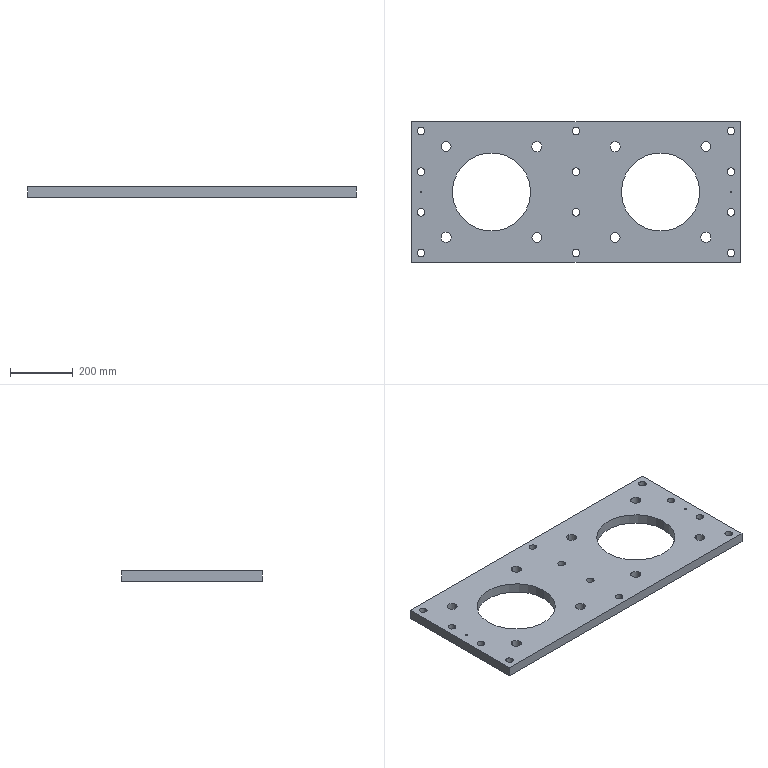Part | SolidWorks | features ICE 3, MirrorPattern 3, CirPattern 1, Extrusion 1, HoleWzd 1 | 1 solid | 54 faces | box 1050 x 450 x 32 mm | volume 11596993 mm3 | cylinder 48 | plane 6 | commonest cylinder face diameters 24 x24 32 x16 6 x4 250 x4